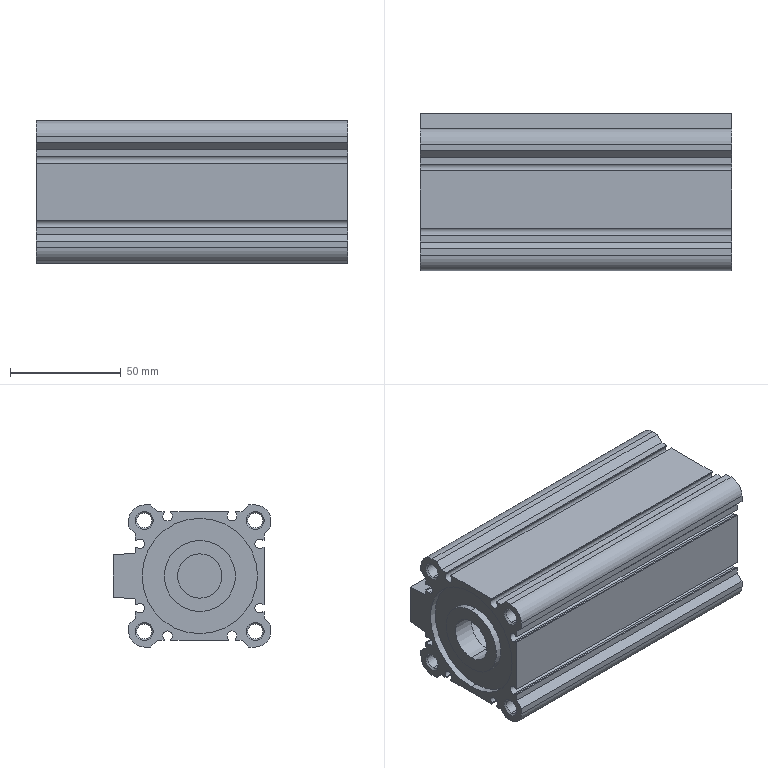Part | STEP file | _CDQ2A50-100-A93(0_0)_BODY.stp | 1 solid | 145 faces | box 140.5 x 71 x 64 mm | volume 265383 mm3 | plane 65 | cylinder 60 | cone 20 | commonest cylinder face diameters 4.26 x18 6.647 x16 8 x8 11.445 x4 14 x4 52 x4